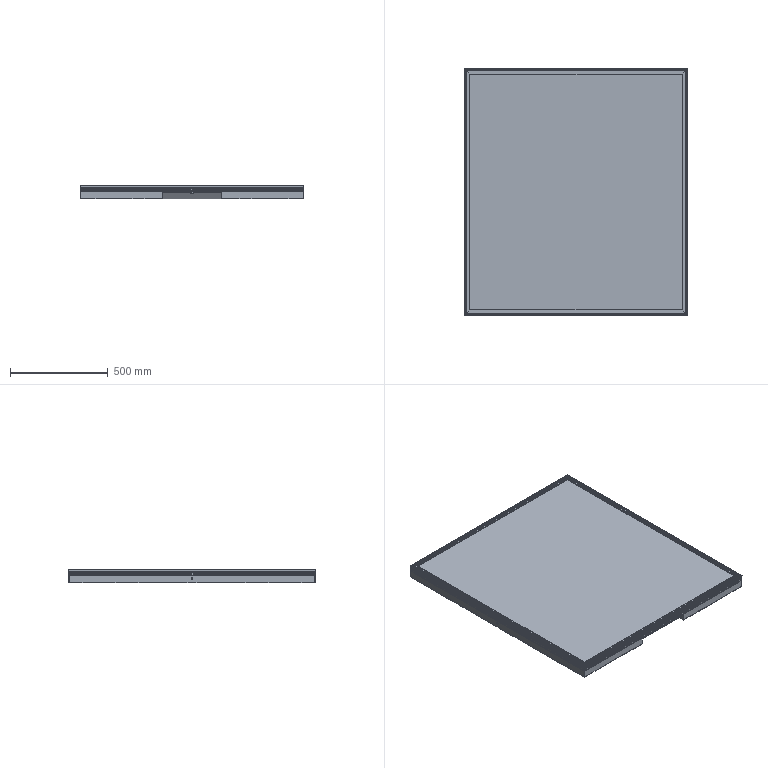Part | SolidWorks | 9 solids | 894 faces | box 1140 x 1260 x 70 mm | volume 25062721 mm3 | plane 590 | cylinder 272 | spline 32 | commonest cylinder face diameters 7 x100 0.4 x67 2.4 x41 11 x28 2 x16 10 x12